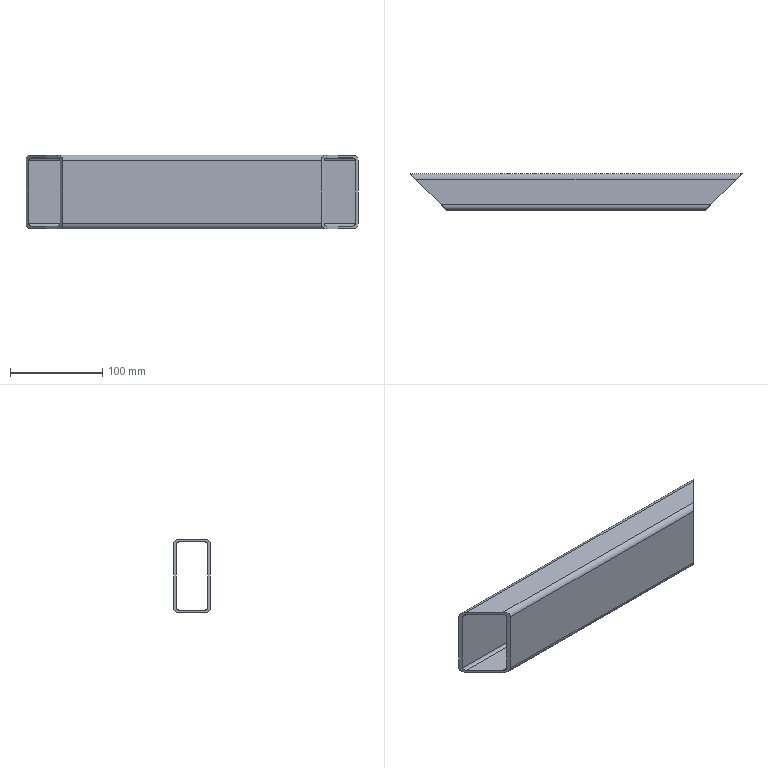Part | STEP file | SN10_002_008-02_TUBO_RETANGULAR | 1 solid | 18 faces | box 360 x 40 x 80 mm | volume 211463 mm3 | plane 10 | cylinder 8 | commonest cylinder face diameters 6 x4 12 x4